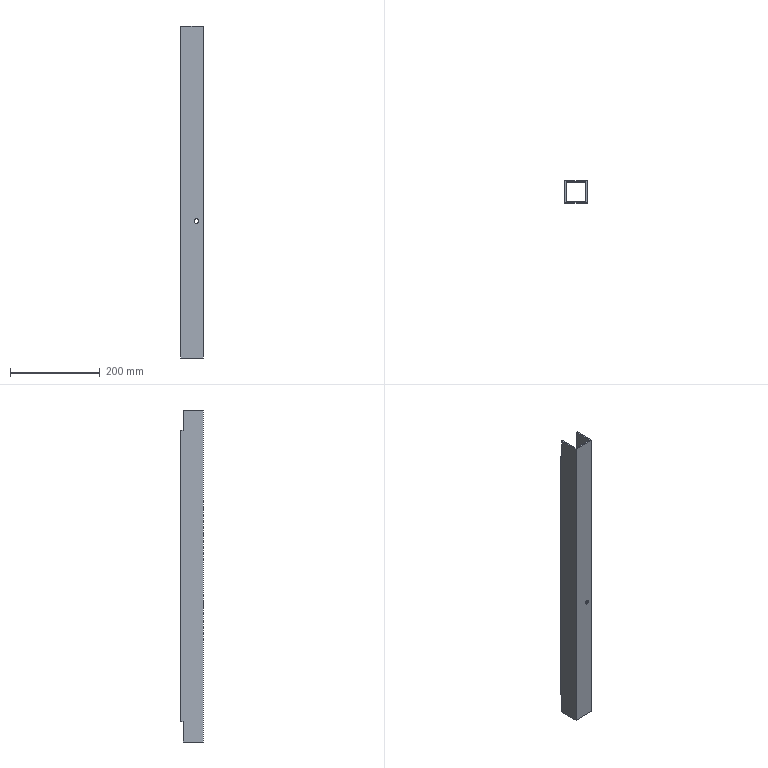Part | SolidWorks | features ICE 6, Cut 3, Extrusion 1 | 1 solid | 20 faces | box 50 x 50 x 740 mm | volume 402309 mm3 | plane 16 | cylinder 4 | commonest cylinder face diameters 10 x4
STEP:
#1=CARTESIAN_POINT('',(35.,0.,325.));
#2=VERTEX_POINT('',#1);
#3=CARTESIAN_POINT('',(35.,0.,335.));
#4=VERTEX_POINT('',#3);
#5=CARTESIAN_POINT('',(35.,0.,330.));
#6=DIRECTION('',(0.,1.,0.));
#7=DIRECTION('',(0.,0.,1.));
#8=AXIS2_PLACEMENT_3D('',#5,#6,#7);
#9=CIRCLE('',#8,5.);
#10=EDGE_CURVE('',#2,#4,#9,.T.);
#11=ORIENTED_EDGE('',*,*,#10,.F.);
#12=CARTESIAN_POINT('',(35.,3.,325.));
#13=VERTEX_POINT('',#12);
#14=CARTESIAN_POINT('',(35.,-44.,325.));
#15=DIRECTION('',(0.,1.,0.));
#16=VECTOR('',#15,1000.);
#17=LINE('',#14,#16);
#18=EDGE_CURVE('',#2,#13,#17,.T.);
#19=ORIENTED_EDGE('',*,*,#18,.T.);
#20=CARTESIAN_POINT('',(35.,3.,335.));
#21=VERTEX_POINT('',#20);
#22=CARTESIAN_POINT('',(35.,3.,330.));
#23=DIRECTION('',(0.,1.,0.));
#24=DIRECTION('',(0.,0.,1.));
#25=AXIS2_PLACEMENT_3D('',#22,#23,#24);
#26=CIRCLE('',#25,5.);
#27=EDGE_CURVE('',#13,#21,#26,.T.);
#28=ORIENTED_EDGE('',*,*,#27,.T.);
#29=CARTESIAN_POINT('',(35.,-44.,335.));
#30=DIRECTION('',(0.,1.,0.));
#31=VECTOR('',#30,1000.);
#32=LINE('',#29,#31);
#33=EDGE_CURVE('',#4,#21,#32,.T.);
#34=ORIENTED_EDGE('',*,*,#33,.F.);
#35=EDGE_LOOP('',(#11,#19,#28,#34));
#36=FACE_OUTER_BOUND('',#35,.T.);
#37=CARTESIAN_POINT('',(35.,-44.,330.));
#38=DIRECTION('',(0.,1.,0.));
#39=DIRECTION('',(0.,0.,1.));
#40=AXIS2_PLACEMENT_3D('',#37,#38,#39);
#41=CYLINDRICAL_SURFACE('',#40,5.);
#42=ADVANCED_FACE('',(#36),#41,.F.);
#43=CARTESIAN_POINT('',(35.,47.,335.));
#44=VERTEX_POINT('',#43);
#45=CARTESIAN_POINT('',(35.,47.,325.));
#46=VERTEX_POINT('',#45);
#47=CARTESIAN_POINT('',(35.,47.,330.));
#48=DIRECTION('',(0.,-1.,0.));
#49=DIRECTION('',(0.,0.,-1.));
#50=AXIS2_PLACEMENT_3D('',#47,#48,#49);
#51=CIRCLE('',#50,5.);
#52=EDGE_CURVE('',#44,#46,#51,.T.);
#53=ORIENTED_EDGE('',*,*,#52,.T.);
#54=CARTESIAN_POINT('',(35.,50.,325.));
#55=VERTEX_POINT('',#54);
#56=CARTESIAN_POINT('',(35.,45.,325.));
#57=DIRECTION('',(0.,1.,0.));
#58=VECTOR('',#57,1000.);
#59=LINE('',#56,#58);
#60=EDGE_CURVE('',#46,#55,#59,.T.);
#61=ORIENTED_EDGE('',*,*,#60,.T.);
#62=CARTESIAN_POINT('',(35.,50.,335.));
#63=VERTEX_POINT('',#62);
#64=CARTESIAN_POINT('',(35.,50.,330.));
#65=DIRECTION('',(0.,1.,0.));
#66=DIRECTION('',(0.,0.,1.));
#67=AXIS2_PLACEMENT_3D('',#64,#65,#66);
#68=CIRCLE('',#67,5.);
#69=EDGE_CURVE('',#55,#63,#68,.T.);
#70=ORIENTED_EDGE('',*,*,#69,.T.);
#71=CARTESIAN_POINT('',(35.,45.,335.));
#72=DIRECTION('',(0.,1.,0.));
#73=VECTOR('',#72,1000.);
#74=LINE('',#71,#73);
#75=EDGE_CURVE('',#44,#63,#74,.T.);
#76=ORIENTED_EDGE('',*,*,#75,.F.);
#77=EDGE_LOOP('',(#53,#61,#70,#76));
#78=FACE_OUTER_BOUND('',#77,.T.);
#79=CARTESIAN_POINT('',(35.,45.,330.));
#80=DIRECTION('',(0.,1.,0.));
#81=DIRECTION('',(0.,0.,1.));
#82=AXIS2_PLACEMENT_3D('',#79,#80,#81);
#83=CYLINDRICAL_SURFACE('',#82,5.);
#84=ADVANCED_FACE('',(#78),#83,.F.);
#85=CARTESIAN_POINT('',(35.,50.,330.));
#86=DIRECTION('',(0.,1.,0.));
#87=DIRECTION('',(0.,0.,1.));
#88=AXIS2_PLACEMENT_3D('',#85,#86,#87);
#89=CIRCLE('',#88,5.);
#90=EDGE_CURVE('',#63,#55,#89,.T.);
#91=ORIENTED_EDGE('',*,*,#90,.F.);
#92=ORIENTED_EDGE('',*,*,#69,.F.);
#93=EDGE_LOOP('',(#91,#92));
#94=FACE_BOUND('',#93,.T.);
#95=CARTESIAN_POINT('',(0.,50.,70.));
#96=VERTEX_POINT('',#95);
#97=CARTESIAN_POINT('',(50.,50.,70.));
#98=VERTEX_POINT('',#97);
#99=CARTESIAN_POINT('',(0.,50.,70.));
#100=DIRECTION('',(1.,0.,0.));
#101=VECTOR('',#100,1000.);
#102=LINE('',#99,#101);
#103=EDGE_CURVE('',#96,#98,#102,.T.);
#104=ORIENTED_EDGE('',*,*,#103,.F.);
#105=CARTESIAN_POINT('',(0.,50.,720.));
#106=VERTEX_POINT('',#105);
#107=CARTESIAN_POINT('',(0.,50.,790.));
#108=DIRECTION('',(0.,0.,-1.));
#109=VECTOR('',#108,1000.);
#110=LINE('',#107,#109);
#111=EDGE_CURVE('',#106,#96,#110,.T.);
#112=ORIENTED_EDGE('',*,*,#111,.F.);
#113=CARTESIAN_POINT('',(50.,50.,720.));
#114=VERTEX_POINT('',#113);
#115=CARTESIAN_POINT('',(50.,50.,720.));
#116=DIRECTION('',(-1.,0.,0.));
#117=VECTOR('',#116,1000.);
#118=LINE('',#115,#117);
#119=EDGE_CURVE('',#114,#106,#118,.T.);
#120=ORIENTED_EDGE('',*,*,#119,.F.);
#121=CARTESIAN_POINT('',(50.,50.,790.));
#122=DIRECTION('',(0.,0.,-1.));
#123=VECTOR('',#122,1000.);
#124=LINE('',#121,#123);
#125=EDGE_CURVE('',#114,#98,#124,.T.);
#126=ORIENTED_EDGE('',*,*,#125,.T.);
#127=EDGE_LOOP('',(#104,#112,#120,#126));
#128=FACE_OUTER_BOUND('',#127,.T.);
#129=CARTESIAN_POINT('',(0.,50.,790.));
#130=DIRECTION('',(0.,-1.,0.));
#131=DIRECTION('',(0.,0.,-1.));
#132=AXIS2_PLACEMENT_3D('',#129,#130,#131);
#133=PLANE('',#132);
#134=ADVANCED_FACE('',(#94,#128),#133,.F.);
#135=ORIENTED_EDGE('',*,*,#52,.F.);
#136=CARTESIAN_POINT('',(35.,47.,330.));
#137=DIRECTION('',(0.,-1.,0.));
#138=DIRECTION('',(0.,0.,-1.));
#139=AXIS2_PLACEMENT_3D('',#136,#137,#138);
#140=CIRCLE('',#139,5.);
#141=EDGE_CURVE('',#46,#44,#140,.T.);
#142=ORIENTED_EDGE('',*,*,#141,.F.);
#143=EDGE_LOOP('',(#135,#142));
#144=FACE_BOUND('',#143,.T.);
#145=CARTESIAN_POINT('',(3.,47.,720.));
#146=VERTEX_POINT('',#145);
#147=CARTESIAN_POINT('',(3.,47.,70.));
#148=VERTEX_POINT('',#147);
#149=CARTESIAN_POINT('',(3.,47.,790.));
#150=DIRECTION('',(0.,0.,-1.));
#151=VECTOR('',#150,1000.);
#152=LINE('',#149,#151);
#153=EDGE_CURVE('',#146,#148,#152,.T.);
#154=ORIENTED_EDGE('',*,*,#153,.T.);
#155=CARTESIAN_POINT('',(47.,47.,70.));
#156=VERTEX_POINT('',#155);
#157=CARTESIAN_POINT('',(47.,47.,70.));
#158=DIRECTION('',(-1.,0.,0.));
#159=VECTOR('',#158,1000.);
#160=LINE('',#157,#159);
#161=EDGE_CURVE('',#156,#148,#160,.T.);
#162=ORIENTED_EDGE('',*,*,#161,.F.);
#163=CARTESIAN_POINT('',(47.,47.,720.));
#164=VERTEX_POINT('',#163);
#165=CARTESIAN_POINT('',(47.,47.,790.));
#166=DIRECTION('',(0.,0.,-1.));
#167=VECTOR('',#166,1000.);
#168=LINE('',#165,#167);
#169=EDGE_CURVE('',#164,#156,#168,.T.);
#170=ORIENTED_EDGE('',*,*,#169,.F.);
#171=CARTESIAN_POINT('',(3.,47.,720.));
#172=DIRECTION('',(1.,0.,0.));
#173=VECTOR('',#172,1000.);
#174=LINE('',#171,#173);
#175=EDGE_CURVE('',#146,#164,#174,.T.);
#176=ORIENTED_EDGE('',*,*,#175,.F.);
#177=EDGE_LOOP('',(#154,#162,#170,#176));
#178=FACE_OUTER_BOUND('',#177,.T.);
#179=CARTESIAN_POINT('',(3.,47.,790.));
#180=DIRECTION('',(0.,-1.,0.));
#181=DIRECTION('',(0.,0.,-1.));
#182=AXIS2_PLACEMENT_3D('',#179,#180,#181);
#183=PLANE('',#182);
#184=ADVANCED_FACE('',(#144,#178),#183,.T.);
#185=CARTESIAN_POINT('',(35.,0.,330.));
#186=DIRECTION('',(0.,1.,0.));
#187=DIRECTION('',(0.,0.,1.));
#188=AXIS2_PLACEMENT_3D('',#185,#186,#187);
#189=CIRCLE('',#188,5.);
#190=EDGE_CURVE('',#4,#2,#189,.T.);
#191=ORIENTED_EDGE('',*,*,#190,.T.);
#192=ORIENTED_EDGE('',*,*,#10,.T.);
#193=EDGE_LOOP('',(#191,#192));
#194=FACE_BOUND('',#193,.T.);
#195=CARTESIAN_POINT('',(50.,0.,25.));
#196=VERTEX_POINT('',#195);
#197=CARTESIAN_POINT('',(0.,0.,25.));
#198=VERTEX_POINT('',#197);
#199=CARTESIAN_POINT('',(50.,0.,25.));
#200=DIRECTION('',(-1.,0.,0.));
#201=VECTOR('',#200,1000.);
#202=LINE('',#199,#201);
#203=EDGE_CURVE('',#196,#198,#202,.T.);
#204=ORIENTED_EDGE('',*,*,#203,.F.);
#205=CARTESIAN_POINT('',(50.,0.,765.));
#206=VERTEX_POINT('',#205);
#207=CARTESIAN_POINT('',(50.,0.,790.));
#208=DIRECTION('',(0.,0.,-1.));
#209=VECTOR('',#208,1000.);
#210=LINE('',#207,#209);
#211=EDGE_CURVE('',#206,#196,#210,.T.);
#212=ORIENTED_EDGE('',*,*,#211,.F.);
#213=CARTESIAN_POINT('',(0.,0.,765.));
#214=VERTEX_POINT('',#213);
#215=CARTESIAN_POINT('',(0.,0.,765.));
#216=DIRECTION('',(1.,0.,0.));
#217=VECTOR('',#216,1000.);
#218=LINE('',#215,#217);
#219=EDGE_CURVE('',#214,#206,#218,.T.);
#220=ORIENTED_EDGE('',*,*,#219,.F.);
#221=CARTESIAN_POINT('',(0.,0.,790.));
#222=DIRECTION('',(0.,0.,-1.));
#223=VECTOR('',#222,1000.);
#224=LINE('',#221,#223);
#225=EDGE_CURVE('',#214,#198,#224,.T.);
#226=ORIENTED_EDGE('',*,*,#225,.T.);
#227=EDGE_LOOP('',(#204,#212,#220,#226));
#228=FACE_OUTER_BOUND('',#227,.T.);
#229=CARTESIAN_POINT('',(50.,0.,790.));
#230=DIRECTION('',(0.,1.,0.));
#231=DIRECTION('',(0.,0.,1.));
#232=AXIS2_PLACEMENT_3D('',#229,#230,#231);
#233=PLANE('',#232);
#234=ADVANCED_FACE('',(#194,#228),#233,.F.);
#235=CARTESIAN_POINT('',(35.,3.,330.));
#236=DIRECTION('',(0.,1.,0.));
#237=DIRECTION('',(0.,0.,1.));
#238=AXIS2_PLACEMENT_3D('',#235,#236,#237);
#239=CIRCLE('',#238,5.);
#240=EDGE_CURVE('',#21,#13,#239,.T.);
#241=ORIENTED_EDGE('',*,*,#240,.F.);
#242=ORIENTED_EDGE('',*,*,#27,.F.);
#243=EDGE_LOOP('',(#241,#242));
#244=FACE_BOUND('',#243,.T.);
#245=CARTESIAN_POINT('',(47.,3.,765.));
#246=VERTEX_POINT('',#245);
#247=CARTESIAN_POINT('',(47.,3.,25.));
#248=VERTEX_POINT('',#247);
#249=CARTESIAN_POINT('',(47.,3.,790.));
#250=DIRECTION('',(0.,0.,-1.));
#251=VECTOR('',#250,1000.);
#252=LINE('',#249,#251);
#253=EDGE_CURVE('',#246,#248,#252,.T.);
#254=ORIENTED_EDGE('',*,*,#253,.T.);
#255=CARTESIAN_POINT('',(3.,3.,25.));
#256=VERTEX_POINT('',#255);
#257=CARTESIAN_POINT('',(3.,3.,25.));
#258=DIRECTION('',(1.,0.,0.));
#259=VECTOR('',#258,1000.);
#260=LINE('',#257,#259);
#261=EDGE_CURVE('',#256,#248,#260,.T.);
#262=ORIENTED_EDGE('',*,*,#261,.F.);
#263=CARTESIAN_POINT('',(3.,3.,765.));
#264=VERTEX_POINT('',#263);
#265=CARTESIAN_POINT('',(3.,3.,790.));
#266=DIRECTION('',(0.,0.,-1.));
#267=VECTOR('',#266,1000.);
#268=LINE('',#265,#267);
#269=EDGE_CURVE('',#264,#256,#268,.T.);
#270=ORIENTED_EDGE('',*,*,#269,.F.);
#271=CARTESIAN_POINT('',(47.,3.,765.));
#272=DIRECTION('',(-1.,0.,0.));
#273=VECTOR('',#272,1000.);
#274=LINE('',#271,#273);
#275=EDGE_CURVE('',#246,#264,#274,.T.);
#276=ORIENTED_EDGE('',*,*,#275,.F.);
#277=EDGE_LOOP('',(#254,#262,#270,#276));
#278=FACE_OUTER_BOUND('',#277,.T.);
#279=CARTESIAN_POINT('',(47.,3.,790.));
#280=DIRECTION('',(0.,1.,0.));
#281=DIRECTION('',(0.,0.,1.));
#282=AXIS2_PLACEMENT_3D('',#279,#280,#281);
#283=PLANE('',#282);
#284=ADVANCED_FACE('',(#244,#278),#283,.T.);
#285=CARTESIAN_POINT('',(50.,45.,70.));
#286=VERTEX_POINT('',#285);
#287=CARTESIAN_POINT('',(50.,45.,25.));
#288=VERTEX_POINT('',#287);
#289=CARTESIAN_POINT('',(50.,45.,45.));
#290=DIRECTION('',(0.,0.,-1.));
#291=VECTOR('',#290,1000.);
#292=LINE('',#289,#291);
#293=EDGE_CURVE('',#286,#288,#292,.T.);
#294=ORIENTED_EDGE('',*,*,#293,.F.);
#295=CARTESIAN_POINT('',(50.,50.,70.));
#296=DIRECTION('',(0.,-1.,0.));
#297=VECTOR('',#296,1000.);
#298=LINE('',#295,#297);
#299=EDGE_CURVE('',#98,#286,#298,.T.);
#300=ORIENTED_EDGE('',*,*,#299,.F.);
#301=ORIENTED_EDGE('',*,*,#125,.F.);
#302=CARTESIAN_POINT('',(50.,45.,720.));
#303=VERTEX_POINT('',#302);
#304=CARTESIAN_POINT('',(50.,45.,720.));
#305=DIRECTION('',(0.,1.,0.));
#306=VECTOR('',#305,1000.);
#307=LINE('',#304,#306);
#308=EDGE_CURVE('',#303,#114,#307,.T.);
#309=ORIENTED_EDGE('',*,*,#308,.F.);
#310=CARTESIAN_POINT('',(50.,45.,765.));
#311=VERTEX_POINT('',#310);
#312=CARTESIAN_POINT('',(50.,45.,695.));
#313=DIRECTION('',(0.,0.,1.));
#314=VECTOR('',#313,1000.);
#315=LINE('',#312,#314);
#316=EDGE_CURVE('',#303,#311,#315,.T.);
#317=ORIENTED_EDGE('',*,*,#316,.T.);
#318=CARTESIAN_POINT('',(50.,0.,765.));
#319=DIRECTION('',(0.,1.,0.));
#320=VECTOR('',#319,1000.);
#321=LINE('',#318,#320);
#322=EDGE_CURVE('',#206,#311,#321,.T.);
#323=ORIENTED_EDGE('',*,*,#322,.F.);
#324=ORIENTED_EDGE('',*,*,#211,.T.);
#325=CARTESIAN_POINT('',(50.,45.,25.));
#326=DIRECTION('',(0.,-1.,0.));
#327=VECTOR('',#326,1000.);
#328=LINE('',#325,#327);
#329=EDGE_CURVE('',#288,#196,#328,.T.);
#330=ORIENTED_EDGE('',*,*,#329,.F.);
#331=EDGE_LOOP('',(#294,#300,#301,#309,#317,#323,#324,#330));
#332=FACE_OUTER_BOUND('',#331,.T.);
#333=CARTESIAN_POINT('',(50.,50.,790.));
#334=DIRECTION('',(-1.,0.,0.));
#335=DIRECTION('',(0.,0.,1.));
#336=AXIS2_PLACEMENT_3D('',#333,#334,#335);
#337=PLANE('',#336);
#338=ADVANCED_FACE('',(#332),#337,.F.);
#339=CARTESIAN_POINT('',(0.,45.,70.));
#340=VERTEX_POINT('',#339);
#341=CARTESIAN_POINT('',(0.,45.,70.));
#342=DIRECTION('',(0.,1.,0.));
#343=VECTOR('',#342,1000.);
#344=LINE('',#341,#343);
#345=EDGE_CURVE('',#340,#96,#344,.T.);
#346=ORIENTED_EDGE('',*,*,#345,.F.);
#347=CARTESIAN_POINT('',(0.,45.,25.));
#348=VERTEX_POINT('',#347);
#349=CARTESIAN_POINT('',(0.,45.,0.));
#350=DIRECTION('',(0.,0.,1.));
#351=VECTOR('',#350,1000.);
#352=LINE('',#349,#351);
#353=EDGE_CURVE('',#348,#340,#352,.T.);
#354=ORIENTED_EDGE('',*,*,#353,.F.);
#355=CARTESIAN_POINT('',(0.,0.,25.));
#356=DIRECTION('',(0.,1.,0.));
#357=VECTOR('',#356,1000.);
#358=LINE('',#355,#357);
#359=EDGE_CURVE('',#198,#348,#358,.T.);
#360=ORIENTED_EDGE('',*,*,#359,.F.);
#361=ORIENTED_EDGE('',*,*,#225,.F.);
#362=CARTESIAN_POINT('',(0.,45.,765.));
#363=VERTEX_POINT('',#362);
#364=CARTESIAN_POINT('',(0.,45.,765.));
#365=DIRECTION('',(0.,-1.,0.));
#366=VECTOR('',#365,1000.);
#367=LINE('',#364,#366);
#368=EDGE_CURVE('',#363,#214,#367,.T.);
#369=ORIENTED_EDGE('',*,*,#368,.F.);
#370=CARTESIAN_POINT('',(0.,45.,720.));
#371=VERTEX_POINT('',#370);
#372=CARTESIAN_POINT('',(0.,45.,695.));
#373=DIRECTION('',(0.,0.,1.));
#374=VECTOR('',#373,1000.);
#375=LINE('',#372,#374);
#376=EDGE_CURVE('',#371,#363,#375,.T.);
#377=ORIENTED_EDGE('',*,*,#376,.F.);
#378=CARTESIAN_POINT('',(0.,50.,720.));
#379=DIRECTION('',(0.,-1.,0.));
#380=VECTOR('',#379,1000.);
#381=LINE('',#378,#380);
#382=EDGE_CURVE('',#106,#371,#381,.T.);
#383=ORIENTED_EDGE('',*,*,#382,.F.);
#384=ORIENTED_EDGE('',*,*,#111,.T.);
#385=EDGE_LOOP('',(#346,#354,#360,#361,#369,#377,#383,#384));
#386=FACE_OUTER_BOUND('',#385,.T.);
#387=CARTESIAN_POINT('',(0.,0.,790.));
#388=DIRECTION('',(1.,0.,0.));
#389=DIRECTION('',(0.,0.,-1.));
#390=AXIS2_PLACEMENT_3D('',#387,#388,#389);
#391=PLANE('',#390);
#392=ADVANCED_FACE('',(#386),#391,.F.);
#393=CARTESIAN_POINT('',(47.,45.,70.));
#394=VERTEX_POINT('',#393);
#395=CARTESIAN_POINT('',(47.,45.,70.));
#396=DIRECTION('',(0.,1.,0.));
#397=VECTOR('',#396,1000.);
#398=LINE('',#395,#397);
#399=EDGE_CURVE('',#394,#156,#398,.T.);
#400=ORIENTED_EDGE('',*,*,#399,.F.);
#401=CARTESIAN_POINT('',(47.,45.,25.));
#402=VERTEX_POINT('',#401);
#403=CARTESIAN_POINT('',(47.,45.,790.));
#404=DIRECTION('',(0.,0.,-1.));
#405=VECTOR('',#404,1000.);
#406=LINE('',#403,#405);
#407=EDGE_CURVE('',#394,#402,#406,.T.);
#408=ORIENTED_EDGE('',*,*,#407,.T.);
#409=CARTESIAN_POINT('',(47.,3.,25.));
#410=DIRECTION('',(0.,1.,0.));
#411=VECTOR('',#410,1000.);
#412=LINE('',#409,#411);
#413=EDGE_CURVE('',#248,#402,#412,.T.);
#414=ORIENTED_EDGE('',*,*,#413,.F.);
#415=ORIENTED_EDGE('',*,*,#253,.F.);
#416=CARTESIAN_POINT('',(47.,45.,765.));
#417=VERTEX_POINT('',#416);
#418=CARTESIAN_POINT('',(47.,45.,765.));
#419=DIRECTION('',(0.,-1.,0.));
#420=VECTOR('',#419,1000.);
#421=LINE('',#418,#420);
#422=EDGE_CURVE('',#417,#246,#421,.T.);
#423=ORIENTED_EDGE('',*,*,#422,.F.);
#424=CARTESIAN_POINT('',(47.,45.,720.));
#425=VERTEX_POINT('',#424);
#426=CARTESIAN_POINT('',(47.,45.,695.));
#427=DIRECTION('',(0.,0.,1.));
#428=VECTOR('',#427,1000.);
#429=LINE('',#426,#428);
#430=EDGE_CURVE('',#425,#417,#429,.T.);
#431=ORIENTED_EDGE('',*,*,#430,.F.);
#432=CARTESIAN_POINT('',(47.,47.,720.));
#433=DIRECTION('',(0.,-1.,0.));
#434=VECTOR('',#433,1000.);
#435=LINE('',#432,#434);
#436=EDGE_CURVE('',#164,#425,#435,.T.);
#437=ORIENTED_EDGE('',*,*,#436,.F.);
#438=ORIENTED_EDGE('',*,*,#169,.T.);
#439=EDGE_LOOP('',(#400,#408,#414,#415,#423,#431,#437,#438));
#440=FACE_OUTER_BOUND('',#439,.T.);
#441=CARTESIAN_POINT('',(47.,47.,790.));
#442=DIRECTION('',(-1.,0.,0.));
#443=DIRECTION('',(0.,0.,1.));
#444=AXIS2_PLACEMENT_3D('',#441,#442,#443);
#445=PLANE('',#444);
#446=ADVANCED_FACE('',(#440),#445,.T.);
#447=CARTESIAN_POINT('',(3.,45.,25.));
#448=VERTEX_POINT('',#447);
#449=CARTESIAN_POINT('',(3.,45.,70.));
#450=VERTEX_POINT('',#449);
#451=CARTESIAN_POINT('',(3.,45.,790.));
#452=DIRECTION('',(0.,0.,1.));
#453=VECTOR('',#452,1000.);
#454=LINE('',#451,#453);
#455=EDGE_CURVE('',#448,#450,#454,.T.);
#456=ORIENTED_EDGE('',*,*,#455,.T.);
#457=CARTESIAN_POINT('',(3.,47.,70.));
#458=DIRECTION('',(0.,-1.,0.));
#459=VECTOR('',#458,1000.);
#460=LINE('',#457,#459);
#461=EDGE_CURVE('',#148,#450,#460,.T.);
#462=ORIENTED_EDGE('',*,*,#461,.F.);
#463=ORIENTED_EDGE('',*,*,#153,.F.);
#464=CARTESIAN_POINT('',(3.,45.,720.));
#465=VERTEX_POINT('',#464);
#466=CARTESIAN_POINT('',(3.,45.,720.));
#467=DIRECTION('',(0.,1.,0.));
#468=VECTOR('',#467,1000.);
#469=LINE('',#466,#468);
#470=EDGE_CURVE('',#465,#146,#469,.T.);
#471=ORIENTED_EDGE('',*,*,#470,.F.);
#472=CARTESIAN_POINT('',(3.,45.,765.));
#473=VERTEX_POINT('',#472);
#474=CARTESIAN_POINT('',(3.,45.,695.));
#475=DIRECTION('',(0.,0.,1.));
#476=VECTOR('',#475,1000.);
#477=LINE('',#474,#476);
#478=EDGE_CURVE('',#465,#473,#477,.T.);
#479=ORIENTED_EDGE('',*,*,#478,.T.);
#480=CARTESIAN_POINT('',(3.,3.,765.));
#481=DIRECTION('',(0.,1.,0.));
#482=VECTOR('',#481,1000.);
#483=LINE('',#480,#482);
#484=EDGE_CURVE('',#264,#473,#483,.T.);
#485=ORIENTED_EDGE('',*,*,#484,.F.);
#486=ORIENTED_EDGE('',*,*,#269,.T.);
#487=CARTESIAN_POINT('',(3.,45.,25.));
#488=DIRECTION('',(0.,-1.,0.));
#489=VECTOR('',#488,1000.);
#490=LINE('',#487,#489);
#491=EDGE_CURVE('',#448,#256,#490,.T.);
#492=ORIENTED_EDGE('',*,*,#491,.F.);
#493=EDGE_LOOP('',(#456,#462,#463,#471,#479,#485,#486,#492));
#494=FACE_OUTER_BOUND('',#493,.T.);
#495=CARTESIAN_POINT('',(3.,3.,790.));
#496=DIRECTION('',(1.,0.,0.));
#497=DIRECTION('',(0.,0.,-1.));
#498=AXIS2_PLACEMENT_3D('',#495,#496,#497);
#499=PLANE('',#498);
#500=ADVANCED_FACE('',(#494),#499,.T.);
#501=ORIENTED_EDGE('',*,*,#293,.T.);
#502=CARTESIAN_POINT('',(47.,45.,25.));
#503=DIRECTION('',(1.,0.,0.));
#504=VECTOR('',#503,1000.);
#505=LINE('',#502,#504);
#506=EDGE_CURVE('',#402,#288,#505,.T.);
#507=ORIENTED_EDGE('',*,*,#506,.F.);
#508=ORIENTED_EDGE('',*,*,#407,.F.);
#509=CARTESIAN_POINT('',(50.,45.,70.));
#510=DIRECTION('',(-1.,0.,0.));
#511=VECTOR('',#510,1000.);
#512=LINE('',#509,#511);
#513=EDGE_CURVE('',#286,#394,#512,.T.);
#514=ORIENTED_EDGE('',*,*,#513,.F.);
#515=EDGE_LOOP('',(#501,#507,#508,#514));
#516=FACE_OUTER_BOUND('',#515,.T.);
#517=CARTESIAN_POINT('',(0.,45.,0.));
#518=DIRECTION('',(0.,1.,0.));
#519=DIRECTION('',(0.,0.,1.));
#520=AXIS2_PLACEMENT_3D('',#517,#518,#519);
#521=PLANE('',#520);
#522=ADVANCED_FACE('',(#516),#521,.T.);
#523=ORIENTED_EDGE('',*,*,#455,.F.);
#524=CARTESIAN_POINT('',(0.,45.,25.));
#525=DIRECTION('',(1.,0.,0.));
#526=VECTOR('',#525,1000.);
#527=LINE('',#524,#526);
#528=EDGE_CURVE('',#348,#448,#527,.T.);
#529=ORIENTED_EDGE('',*,*,#528,.F.);
#530=ORIENTED_EDGE('',*,*,#353,.T.);
#531=CARTESIAN_POINT('',(3.,45.,70.));
#532=DIRECTION('',(-1.,0.,0.));
#533=VECTOR('',#532,1000.);
#534=LINE('',#531,#533);
#535=EDGE_CURVE('',#450,#340,#534,.T.);
#536=ORIENTED_EDGE('',*,*,#535,.F.);
#537=EDGE_LOOP('',(#523,#529,#530,#536));
#538=FACE_OUTER_BOUND('',#537,.T.);
#539=CARTESIAN_POINT('',(0.,45.,0.));
#540=DIRECTION('',(0.,1.,0.));
#541=DIRECTION('',(0.,0.,1.));
#542=AXIS2_PLACEMENT_3D('',#539,#540,#541);
#543=PLANE('',#542);
#544=ADVANCED_FACE('',(#538),#543,.T.);
#545=CARTESIAN_POINT('',(0.,45.,720.));
#546=DIRECTION('',(1.,0.,0.));
#547=VECTOR('',#546,1000.);
#548=LINE('',#545,#547);
#549=EDGE_CURVE('',#371,#465,#548,.T.);
#550=ORIENTED_EDGE('',*,*,#549,.F.);
#551=ORIENTED_EDGE('',*,*,#376,.T.);
#552=CARTESIAN_POINT('',(3.,45.,765.));
#553=DIRECTION('',(-1.,0.,0.));
#554=VECTOR('',#553,1000.);
#555=LINE('',#552,#554);
#556=EDGE_CURVE('',#473,#363,#555,.T.);
#557=ORIENTED_EDGE('',*,*,#556,.F.);
#558=ORIENTED_EDGE('',*,*,#478,.F.);
#559=EDGE_LOOP('',(#550,#551,#557,#558));
#560=FACE_OUTER_BOUND('',#559,.T.);
#561=CARTESIAN_POINT('',(0.,45.,695.));
#562=DIRECTION('',(0.,-1.,0.));
#563=DIRECTION('',(0.,0.,-1.));
#564=AXIS2_PLACEMENT_3D('',#561,#562,#563);
#565=PLANE('',#564);
#566=ADVANCED_FACE('',(#560),#565,.F.);
#567=CARTESIAN_POINT('',(47.,45.,720.));
#568=DIRECTION('',(1.,0.,0.));
#569=VECTOR('',#568,1000.);
#570=LINE('',#567,#569);
#571=EDGE_CURVE('',#425,#303,#570,.T.);
#572=ORIENTED_EDGE('',*,*,#571,.F.);
#573=ORIENTED_EDGE('',*,*,#430,.T.);
#574=CARTESIAN_POINT('',(50.,45.,765.));
#575=DIRECTION('',(-1.,0.,0.));
#576=VECTOR('',#575,1000.);
#577=LINE('',#574,#576);
#578=EDGE_CURVE('',#311,#417,#577,.T.);
#579=ORIENTED_EDGE('',*,*,#578,.F.);
#580=ORIENTED_EDGE('',*,*,#316,.F.);
#581=EDGE_LOOP('',(#572,#573,#579,#580));
#582=FACE_OUTER_BOUND('',#581,.T.);
#583=CARTESIAN_POINT('',(47.,45.,695.));
#584=DIRECTION('',(0.,-1.,0.));
#585=DIRECTION('',(0.,0.,-1.));
#586=AXIS2_PLACEMENT_3D('',#583,#584,#585);
#587=PLANE('',#586);
#588=ADVANCED_FACE('',(#582),#587,.F.);
#589=ORIENTED_EDGE('',*,*,#60,.F.);
#590=ORIENTED_EDGE('',*,*,#141,.T.);
#591=ORIENTED_EDGE('',*,*,#75,.T.);
#592=ORIENTED_EDGE('',*,*,#90,.T.);
#593=EDGE_LOOP('',(#589,#590,#591,#592));
#594=FACE_OUTER_BOUND('',#593,.T.);
#595=CARTESIAN_POINT('',(35.,45.,330.));
#596=DIRECTION('',(0.,1.,0.));
#597=DIRECTION('',(0.,0.,1.));
#598=AXIS2_PLACEMENT_3D('',#595,#596,#597);
#599=CYLINDRICAL_SURFACE('',#598,5.);
#600=ADVANCED_FACE('',(#594),#599,.F.);
#601=ORIENTED_EDGE('',*,*,#470,.T.);
#602=ORIENTED_EDGE('',*,*,#175,.T.);
#603=ORIENTED_EDGE('',*,*,#436,.T.);
#604=ORIENTED_EDGE('',*,*,#571,.T.);
#605=ORIENTED_EDGE('',*,*,#308,.T.);
#606=ORIENTED_EDGE('',*,*,#119,.T.);
#607=ORIENTED_EDGE('',*,*,#382,.T.);
#608=ORIENTED_EDGE('',*,*,#549,.T.);
#609=EDGE_LOOP('',(#601,#602,#603,#604,#605,#606,#607,#608));
#610=FACE_OUTER_BOUND('',#609,.T.);
#611=CARTESIAN_POINT('',(0.,0.,720.));
#612=DIRECTION('',(0.,0.,-1.));
#613=DIRECTION('',(-1.,0.,0.));
#614=AXIS2_PLACEMENT_3D('',#611,#612,#613);
#615=PLANE('',#614);
#616=ADVANCED_FACE('',(#610),#615,.F.);
#617=ORIENTED_EDGE('',*,*,#368,.T.);
#618=ORIENTED_EDGE('',*,*,#219,.T.);
#619=ORIENTED_EDGE('',*,*,#322,.T.);
#620=ORIENTED_EDGE('',*,*,#578,.T.);
#621=ORIENTED_EDGE('',*,*,#422,.T.);
#622=ORIENTED_EDGE('',*,*,#275,.T.);
#623=ORIENTED_EDGE('',*,*,#484,.T.);
#624=ORIENTED_EDGE('',*,*,#556,.T.);
#625=EDGE_LOOP('',(#617,#618,#619,#620,#621,#622,#623,#624));
#626=FACE_OUTER_BOUND('',#625,.T.);
#627=CARTESIAN_POINT('',(0.,0.,765.));
#628=DIRECTION('',(0.,0.,1.));
#629=DIRECTION('',(1.,0.,0.));
#630=AXIS2_PLACEMENT_3D('',#627,#628,#629);
#631=PLANE('',#630);
#632=ADVANCED_FACE('',(#626),#631,.T.);
#633=ORIENTED_EDGE('',*,*,#203,.T.);
#634=ORIENTED_EDGE('',*,*,#359,.T.);
#635=ORIENTED_EDGE('',*,*,#528,.T.);
#636=ORIENTED_EDGE('',*,*,#491,.T.);
#637=ORIENTED_EDGE('',*,*,#261,.T.);
#638=ORIENTED_EDGE('',*,*,#413,.T.);
#639=ORIENTED_EDGE('',*,*,#506,.T.);
#640=ORIENTED_EDGE('',*,*,#329,.T.);
#641=EDGE_LOOP('',(#633,#634,#635,#636,#637,#638,#639,#640));
#642=FACE_OUTER_BOUND('',#641,.T.);
#643=CARTESIAN_POINT('',(0.,0.,25.));
#644=DIRECTION('',(0.,0.,-1.));
#645=DIRECTION('',(-1.,0.,0.));
#646=AXIS2_PLACEMENT_3D('',#643,#644,#645);
#647=PLANE('',#646);
#648=ADVANCED_FACE('',(#642),#647,.T.);
#649=ORIENTED_EDGE('',*,*,#513,.T.);
#650=ORIENTED_EDGE('',*,*,#399,.T.);
#651=ORIENTED_EDGE('',*,*,#161,.T.);
#652=ORIENTED_EDGE('',*,*,#461,.T.);
#653=ORIENTED_EDGE('',*,*,#535,.T.);
#654=ORIENTED_EDGE('',*,*,#345,.T.);
#655=ORIENTED_EDGE('',*,*,#103,.T.);
#656=ORIENTED_EDGE('',*,*,#299,.T.);
#657=EDGE_LOOP('',(#649,#650,#651,#652,#653,#654,#655,#656));
#658=FACE_OUTER_BOUND('',#657,.T.);
#659=CARTESIAN_POINT('',(0.,0.,70.));
#660=DIRECTION('',(0.,0.,-1.));
#661=DIRECTION('',(-1.,0.,0.));
#662=AXIS2_PLACEMENT_3D('',#659,#660,#661);
#663=PLANE('',#662);
#664=ADVANCED_FACE('',(#658),#663,.T.);
#665=ORIENTED_EDGE('',*,*,#18,.F.);
#666=ORIENTED_EDGE('',*,*,#190,.F.);
#667=ORIENTED_EDGE('',*,*,#33,.T.);
#668=ORIENTED_EDGE('',*,*,#240,.T.);
#669=EDGE_LOOP('',(#665,#666,#667,#668));
#670=FACE_OUTER_BOUND('',#669,.T.);
#671=CARTESIAN_POINT('',(35.,-44.,330.));
#672=DIRECTION('',(0.,1.,0.));
#673=DIRECTION('',(0.,0.,1.));
#674=AXIS2_PLACEMENT_3D('',#671,#672,#673);
#675=CYLINDRICAL_SURFACE('',#674,5.);
#676=ADVANCED_FACE('',(#670),#675,.F.);
#677=CLOSED_SHELL('',(#42,#84,#134,#184,#234,#284,#338,#392,#446,#500,#522,#544,#566,#588,#600,#616,#632,#648,#664,#676));
#678=MANIFOLD_SOLID_BREP('',#677);
#679=CARTESIAN_POINT('',(0.,0.,0.));
#680=DIRECTION('',(0.,0.,1.));
#681=DIRECTION('',(1.,0.,0.));
#682=AXIS2_PLACEMENT_3D('',#679,#680,#681);
#683=(LENGTH_UNIT()NAMED_UNIT(*)SI_UNIT(.MILLI.,.METRE.));
#684=UNCERTAINTY_MEASURE_WITH_UNIT(LENGTH_MEASURE(0.00001),#683,'','');
#685=(NAMED_UNIT(*)PLANE_ANGLE_UNIT()SI_UNIT($,.RADIAN.));
#686=(NAMED_UNIT(*)SI_UNIT($,.STERADIAN.)SOLID_ANGLE_UNIT());
#687=(GEOMETRIC_REPRESENTATION_CONTEXT(3)GLOBAL_UNCERTAINTY_ASSIGNED_CONTEXT((#684))GLOBAL_UNIT_ASSIGNED_CONTEXT((#683,#685,#686))REPRESENTATION_CONTEXT('',''));
#688=ADVANCED_BREP_SHAPE_REPRESENTATION('',(#678,#682),#687);